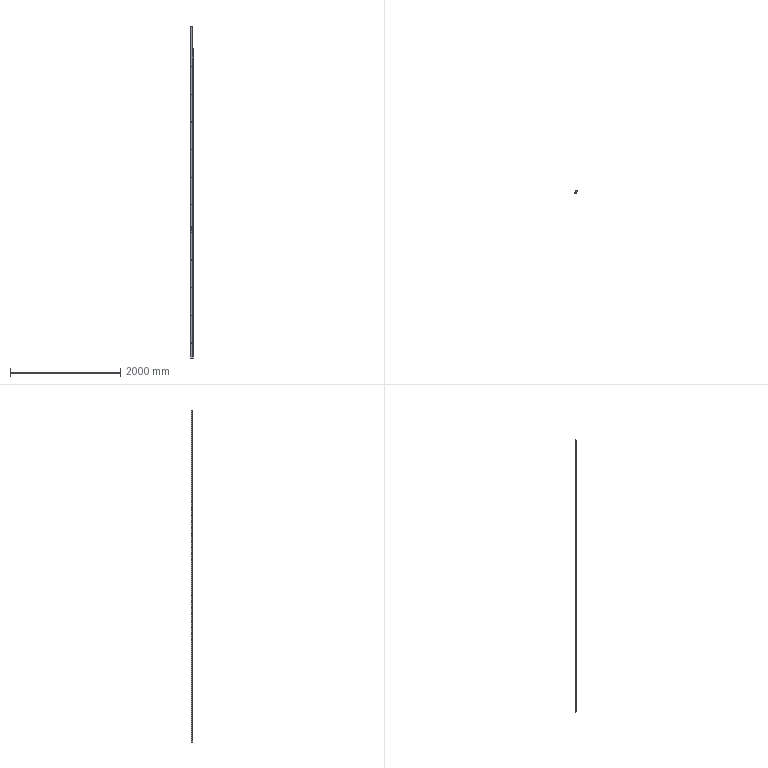Part | STEP file | ASND-0110-5.1 | 1 solid | 68 faces | box 44.772 x 36.1 x 6010 mm | volume 4157112 mm3 | plane 42 | cylinder 26 | commonest cylinder face diameters 4.595 x22 20 x4